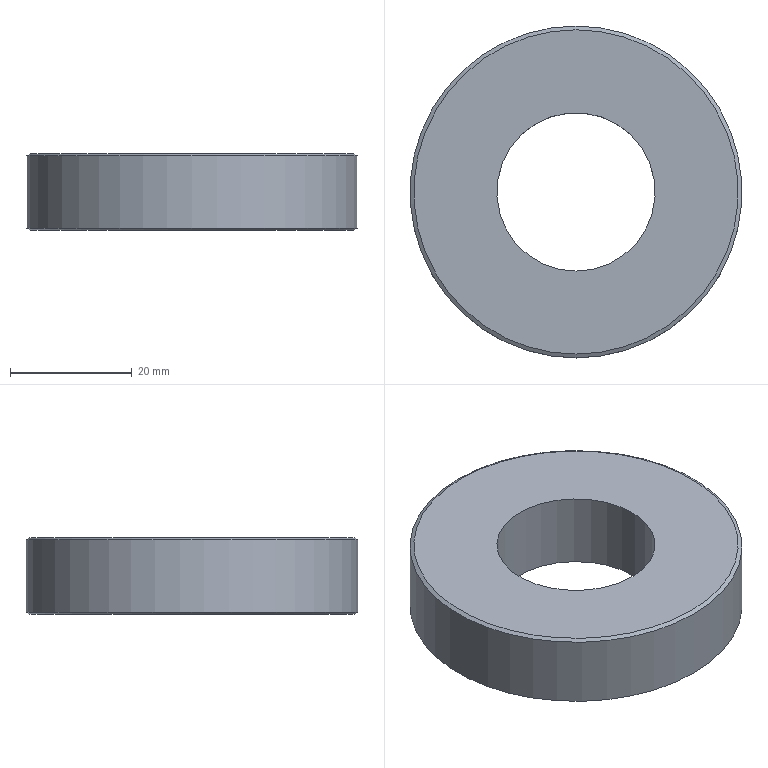Part | NX | features BODY_5003_007_C-SCPW55-12-15 2 | 1 solid | 6 faces | box 54.5 x 54.5 x 12.6 mm | volume 22666 mm3 | cylinder 2 | plane 2 | cone 2 | commonest cylinder face diameters 26 x1 54.5 x1
STEP:
#1=CARTESIAN_POINT('',(158.525,-349.25,-290.56));
#2=VERTEX_POINT('',#1);
#3=CARTESIAN_POINT('',(158.525,-322.,-290.56));
#4=DIRECTION('',(0.,0.,-1.));
#5=DIRECTION('',(0.,-1.,0.));
#6=AXIS2_PLACEMENT_3D('',#3,#4,#5);
#7=CIRCLE('',#6,27.25);
#8=EDGE_CURVE('',#2,#2,#7,.T.);
#9=ORIENTED_EDGE('',*,*,#8,.T.);
#10=EDGE_LOOP('',(#9));
#11=FACE_BOUND('',#10,.T.);
#12=CARTESIAN_POINT('',(158.525,-294.75,-302.44));
#13=VERTEX_POINT('',#12);
#14=CARTESIAN_POINT('',(158.525,-322.,-302.44));
#15=DIRECTION('',(0.,0.,1.));
#16=DIRECTION('',(0.,1.,0.));
#17=AXIS2_PLACEMENT_3D('',#14,#15,#16);
#18=CIRCLE('',#17,27.25);
#19=EDGE_CURVE('',#13,#13,#18,.T.);
#20=ORIENTED_EDGE('',*,*,#19,.T.);
#21=EDGE_LOOP('',(#20));
#22=FACE_BOUND('',#21,.T.);
#23=CARTESIAN_POINT('',(158.525,-322.,-303.43));
#24=DIRECTION('',(0.,0.,-1.));
#25=DIRECTION('',(0.,-1.,0.));
#26=AXIS2_PLACEMENT_3D('',#23,#24,#25);
#27=CYLINDRICAL_SURFACE('',#26,27.25);
#28=ADVANCED_FACE('',(#11,#22),#27,.T.);
#29=CARTESIAN_POINT('',(158.525,-348.626,-290.2));
#30=VERTEX_POINT('',#29);
#31=CARTESIAN_POINT('',(158.525,-322.,-290.2));
#32=DIRECTION('',(0.,0.,-1.));
#33=DIRECTION('',(0.,-1.,0.));
#34=AXIS2_PLACEMENT_3D('',#31,#32,#33);
#35=CIRCLE('',#34,26.626);
#36=EDGE_CURVE('',#30,#30,#35,.F.);
#37=ORIENTED_EDGE('',*,*,#36,.T.);
#38=EDGE_LOOP('',(#37));
#39=FACE_BOUND('',#38,.T.);
#40=CARTESIAN_POINT('',(158.525,-335.,-290.2));
#41=VERTEX_POINT('',#40);
#42=CARTESIAN_POINT('',(158.525,-322.,-290.2));
#43=DIRECTION('',(0.,0.,-1.));
#44=DIRECTION('',(0.,-1.,0.));
#45=AXIS2_PLACEMENT_3D('',#42,#43,#44);
#46=CIRCLE('',#45,13.);
#47=EDGE_CURVE('',#41,#41,#46,.T.);
#48=ORIENTED_EDGE('',*,*,#47,.T.);
#49=EDGE_LOOP('',(#48));
#50=FACE_BOUND('',#49,.T.);
#51=CARTESIAN_POINT('',(131.275,-322.,-290.2));
#52=DIRECTION('',(0.,0.,-1.));
#53=DIRECTION('',(0.,-1.,0.));
#54=AXIS2_PLACEMENT_3D('',#51,#52,#53);
#55=PLANE('',#54);
#56=ADVANCED_FACE('',(#39,#50),#55,.F.);
#57=ORIENTED_EDGE('',*,*,#47,.F.);
#58=EDGE_LOOP('',(#57));
#59=FACE_BOUND('',#58,.T.);
#60=CARTESIAN_POINT('',(158.525,-335.,-302.8));
#61=VERTEX_POINT('',#60);
#62=CARTESIAN_POINT('',(158.525,-322.,-302.8));
#63=DIRECTION('',(0.,0.,-1.));
#64=DIRECTION('',(0.,-1.,0.));
#65=AXIS2_PLACEMENT_3D('',#62,#63,#64);
#66=CIRCLE('',#65,13.);
#67=EDGE_CURVE('',#61,#61,#66,.T.);
#68=ORIENTED_EDGE('',*,*,#67,.T.);
#69=EDGE_LOOP('',(#68));
#70=FACE_BOUND('',#69,.T.);
#71=CARTESIAN_POINT('',(158.525,-322.,-303.43));
#72=DIRECTION('',(0.,0.,-1.));
#73=DIRECTION('',(0.,-1.,0.));
#74=AXIS2_PLACEMENT_3D('',#71,#72,#73);
#75=CYLINDRICAL_SURFACE('',#74,13.);
#76=ADVANCED_FACE('',(#59,#70),#75,.F.);
#77=CARTESIAN_POINT('',(158.525,-295.374,-302.8));
#78=VERTEX_POINT('',#77);
#79=CARTESIAN_POINT('',(158.525,-322.,-302.8));
#80=DIRECTION('',(0.,0.,1.));
#81=DIRECTION('',(0.,1.,0.));
#82=AXIS2_PLACEMENT_3D('',#79,#80,#81);
#83=CIRCLE('',#82,26.626);
#84=EDGE_CURVE('',#78,#78,#83,.F.);
#85=ORIENTED_EDGE('',*,*,#84,.T.);
#86=EDGE_LOOP('',(#85));
#87=FACE_BOUND('',#86,.T.);
#88=ORIENTED_EDGE('',*,*,#67,.F.);
#89=EDGE_LOOP('',(#88));
#90=FACE_BOUND('',#89,.T.);
#91=CARTESIAN_POINT('',(145.525,-322.,-302.8));
#92=DIRECTION('',(0.,0.,1.));
#93=DIRECTION('',(0.,1.,0.));
#94=AXIS2_PLACEMENT_3D('',#91,#92,#93);
#95=PLANE('',#94);
#96=ADVANCED_FACE('',(#87,#90),#95,.F.);
#97=ORIENTED_EDGE('',*,*,#36,.F.);
#98=EDGE_LOOP('',(#97));
#99=FACE_BOUND('',#98,.T.);
#100=ORIENTED_EDGE('',*,*,#8,.F.);
#101=EDGE_LOOP('',(#100));
#102=FACE_BOUND('',#101,.T.);
#103=CARTESIAN_POINT('',(158.525,-322.,-290.56));
#104=DIRECTION('',(0.,0.,-1.));
#105=DIRECTION('',(0.,-1.,0.));
#106=AXIS2_PLACEMENT_3D('',#103,#104,#105);
#107=CONICAL_SURFACE('',#106,27.25,1.047);
#108=ADVANCED_FACE('',(#99,#102),#107,.T.);
#109=ORIENTED_EDGE('',*,*,#19,.F.);
#110=EDGE_LOOP('',(#109));
#111=FACE_BOUND('',#110,.T.);
#112=ORIENTED_EDGE('',*,*,#84,.F.);
#113=EDGE_LOOP('',(#112));
#114=FACE_BOUND('',#113,.T.);
#115=CARTESIAN_POINT('',(158.525,-322.,-302.8));
#116=DIRECTION('',(0.,0.,1.));
#117=DIRECTION('',(0.,1.,0.));
#118=AXIS2_PLACEMENT_3D('',#115,#116,#117);
#119=CONICAL_SURFACE('',#118,26.626,1.047);
#120=ADVANCED_FACE('',(#111,#114),#119,.T.);
#121=CLOSED_SHELL('',(#28,#56,#76,#96,#108,#120));
#122=MANIFOLD_SOLID_BREP('',#121);
#123=(LENGTH_UNIT()NAMED_UNIT(*)SI_UNIT(.MILLI.,.METRE.));
#124=UNCERTAINTY_MEASURE_WITH_UNIT(LENGTH_MEASURE(0.00001),#123,'','');
#125=(NAMED_UNIT(*)PLANE_ANGLE_UNIT()SI_UNIT($,.RADIAN.));
#126=(NAMED_UNIT(*)SI_UNIT($,.STERADIAN.)SOLID_ANGLE_UNIT());
#127=(GEOMETRIC_REPRESENTATION_CONTEXT(3)GLOBAL_UNCERTAINTY_ASSIGNED_CONTEXT((#124))GLOBAL_UNIT_ASSIGNED_CONTEXT((#123,#125,#126))REPRESENTATION_CONTEXT('',''));
#128=ADVANCED_BREP_SHAPE_REPRESENTATION('',(#122),#127);